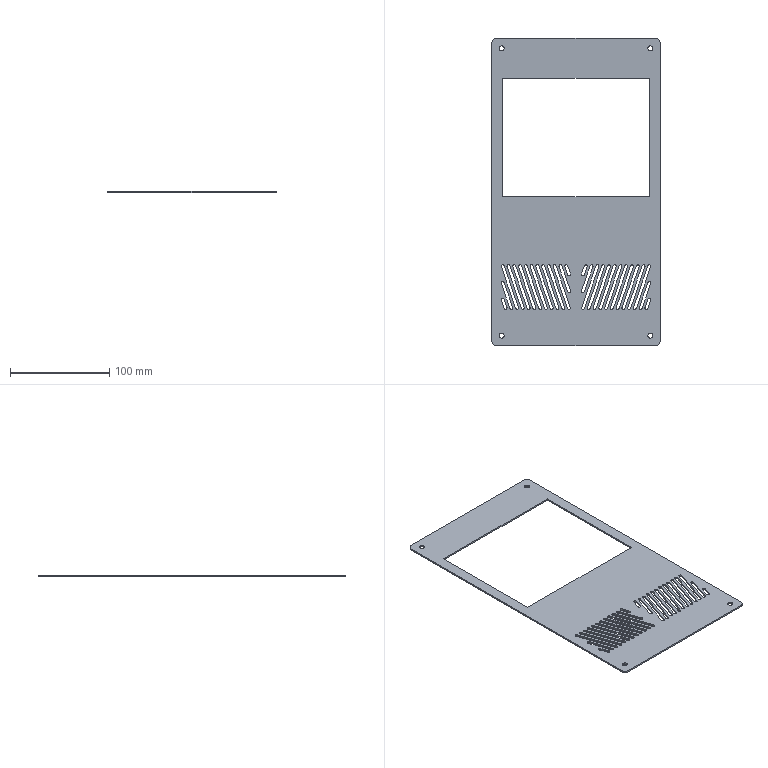Part | STEP file | HESS-408-70-15W-W-34-front control panel | 1 solid | 162 faces | box 170 x 310 x 1.5 mm | volume 47327 mm3 | cylinder 96 | plane 66 | commonest cylinder face diameters 3 x84 5 x8 10 x4